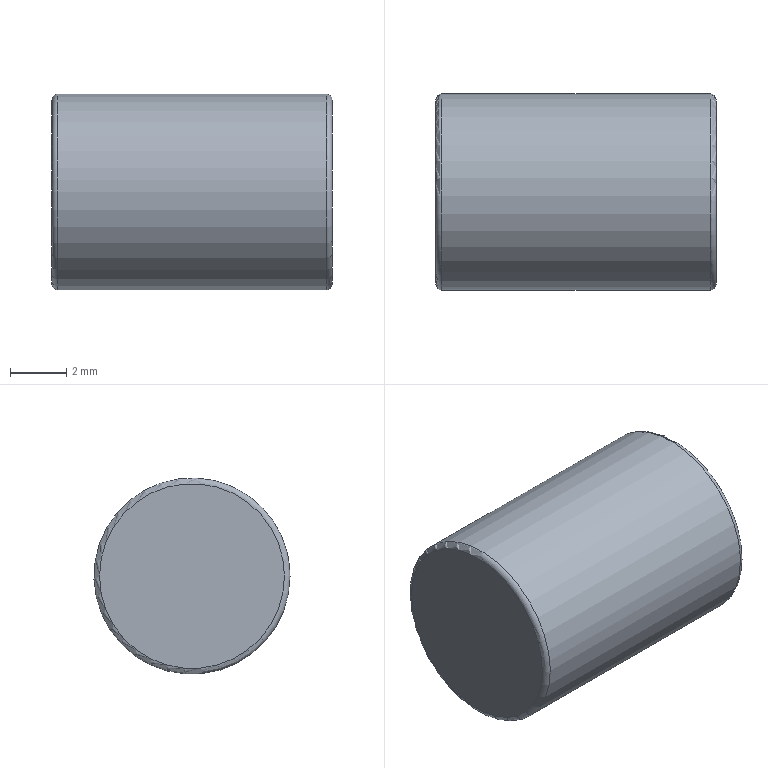Part | STEP file | Part [15] | 1 solid | 5 faces | box 10 x 7 x 7 mm | volume 384.472 mm3 | plane 2 | torus 2 | cylinder 1 | commonest cylinder face diameters 7 x1
STEP:
#1=CARTESIAN_POINT('',(-5.,-126.094,0.));
#2=VERTEX_POINT('',#1);
#3=CARTESIAN_POINT('',(-5.,-122.794,0.));
#4=DIRECTION('',(-1.,0.,0.));
#5=DIRECTION('',(0.,-1.,0.));
#6=AXIS2_PLACEMENT_3D('',#3,#4,#5);
#7=CIRCLE('',#6,3.3);
#8=EDGE_CURVE('',#2,#2,#7,.T.);
#9=ORIENTED_EDGE('',*,*,#8,.T.);
#10=EDGE_LOOP('',(#9));
#11=FACE_BOUND('',#10,.T.);
#12=CARTESIAN_POINT('',(-5.,-122.794,0.));
#13=DIRECTION('',(1.,0.,0.));
#14=DIRECTION('',(0.,0.,1.));
#15=AXIS2_PLACEMENT_3D('',#12,#13,#14);
#16=PLANE('',#15);
#17=ADVANCED_FACE('',(#11),#16,.F.);
#18=CARTESIAN_POINT('',(-4.8,-126.294,0.));
#19=VERTEX_POINT('',#18);
#20=CARTESIAN_POINT('',(-4.8,-126.294,0.));
#21=CARTESIAN_POINT('',(-4.8,-126.294,-0.07332));
#22=CARTESIAN_POINT('',(-4.8,-126.289,-0.2199));
#23=CARTESIAN_POINT('',(-4.8,-126.269,-0.439));
#24=CARTESIAN_POINT('',(-4.8,-126.234,-0.6564));
#25=CARTESIAN_POINT('',(-4.8,-126.186,-0.8711));
#26=CARTESIAN_POINT('',(-4.8,-126.125,-1.082));
#27=CARTESIAN_POINT('',(-4.8,-126.05,-1.289));
#28=CARTESIAN_POINT('',(-4.8,-125.963,-1.491));
#29=CARTESIAN_POINT('',(-4.8,-125.863,-1.687));
#30=CARTESIAN_POINT('',(-4.8,-125.751,-1.877));
#31=CARTESIAN_POINT('',(-4.8,-125.627,-2.059));
#32=CARTESIAN_POINT('',(-4.8,-125.492,-2.233));
#33=CARTESIAN_POINT('',(-4.8,-125.347,-2.398));
#34=CARTESIAN_POINT('',(-4.8,-125.191,-2.553));
#35=CARTESIAN_POINT('',(-4.8,-125.026,-2.699));
#36=CARTESIAN_POINT('',(-4.8,-124.852,-2.834));
#37=CARTESIAN_POINT('',(-4.8,-124.67,-2.957));
#38=CARTESIAN_POINT('',(-4.8,-124.481,-3.069));
#39=CARTESIAN_POINT('',(-4.8,-124.285,-3.169));
#40=CARTESIAN_POINT('',(-4.8,-124.083,-3.257));
#41=CARTESIAN_POINT('',(-4.8,-123.876,-3.331));
#42=CARTESIAN_POINT('',(-4.8,-123.664,-3.392));
#43=CARTESIAN_POINT('',(-4.8,-123.45,-3.44));
#44=CARTESIAN_POINT('',(-4.8,-123.232,-3.475));
#45=CARTESIAN_POINT('',(-4.8,-123.013,-3.495));
#46=CARTESIAN_POINT('',(-4.8,-122.793,-3.502));
#47=CARTESIAN_POINT('',(-4.8,-122.573,-3.495));
#48=CARTESIAN_POINT('',(-4.8,-122.354,-3.475));
#49=CARTESIAN_POINT('',(-4.8,-122.137,-3.44));
#50=CARTESIAN_POINT('',(-4.8,-121.922,-3.392));
#51=CARTESIAN_POINT('',(-4.8,-121.711,-3.331));
#52=CARTESIAN_POINT('',(-4.8,-121.504,-3.256));
#53=CARTESIAN_POINT('',(-4.8,-121.302,-3.169));
#54=CARTESIAN_POINT('',(-4.8,-121.106,-3.069));
#55=CARTESIAN_POINT('',(-4.8,-120.916,-2.956));
#56=CARTESIAN_POINT('',(-4.8,-120.734,-2.833));
#57=CARTESIAN_POINT('',(-4.8,-120.561,-2.698));
#58=CARTESIAN_POINT('',(-4.8,-120.396,-2.552));
#59=CARTESIAN_POINT('',(-4.8,-120.24,-2.397));
#60=CARTESIAN_POINT('',(-4.8,-120.095,-2.231));
#61=CARTESIAN_POINT('',(-4.8,-119.96,-2.057));
#62=CARTESIAN_POINT('',(-4.8,-119.836,-1.875));
#63=CARTESIAN_POINT('',(-4.8,-119.724,-1.686));
#64=CARTESIAN_POINT('',(-4.8,-119.624,-1.49));
#65=CARTESIAN_POINT('',(-4.8,-119.537,-1.288));
#66=CARTESIAN_POINT('',(-4.8,-119.463,-1.081));
#67=CARTESIAN_POINT('',(-4.8,-119.401,-0.8694));
#68=CARTESIAN_POINT('',(-4.8,-119.353,-0.6546));
#69=CARTESIAN_POINT('',(-4.8,-119.319,-0.4373));
#70=CARTESIAN_POINT('',(-4.8,-119.299,-0.2188));
#71=CARTESIAN_POINT('',(-4.8,-119.294,-0.07273));
#72=CARTESIAN_POINT('',(-4.8,-119.294,0.));
#73=CARTESIAN_POINT('',(-4.8,-119.294,0.07332));
#74=CARTESIAN_POINT('',(-4.8,-119.299,0.2199));
#75=CARTESIAN_POINT('',(-4.8,-119.319,0.439));
#76=CARTESIAN_POINT('',(-4.8,-119.354,0.6564));
#77=CARTESIAN_POINT('',(-4.8,-119.402,0.8711));
#78=CARTESIAN_POINT('',(-4.8,-119.463,1.082));
#79=CARTESIAN_POINT('',(-4.8,-119.538,1.289));
#80=CARTESIAN_POINT('',(-4.8,-119.625,1.491));
#81=CARTESIAN_POINT('',(-4.8,-119.725,1.687));
#82=CARTESIAN_POINT('',(-4.8,-119.837,1.877));
#83=CARTESIAN_POINT('',(-4.8,-119.961,2.059));
#84=CARTESIAN_POINT('',(-4.8,-120.096,2.233));
#85=CARTESIAN_POINT('',(-4.8,-120.241,2.398));
#86=CARTESIAN_POINT('',(-4.8,-120.397,2.553));
#87=CARTESIAN_POINT('',(-4.8,-120.562,2.699));
#88=CARTESIAN_POINT('',(-4.8,-120.736,2.834));
#89=CARTESIAN_POINT('',(-4.8,-120.918,2.957));
#90=CARTESIAN_POINT('',(-4.8,-121.107,3.069));
#91=CARTESIAN_POINT('',(-4.8,-121.303,3.169));
#92=CARTESIAN_POINT('',(-4.8,-121.505,3.257));
#93=CARTESIAN_POINT('',(-4.8,-121.712,3.331));
#94=CARTESIAN_POINT('',(-4.8,-121.924,3.392));
#95=CARTESIAN_POINT('',(-4.8,-122.138,3.44));
#96=CARTESIAN_POINT('',(-4.8,-122.356,3.475));
#97=CARTESIAN_POINT('',(-4.8,-122.575,3.495));
#98=CARTESIAN_POINT('',(-4.8,-122.795,3.502));
#99=CARTESIAN_POINT('',(-4.8,-123.015,3.495));
#100=CARTESIAN_POINT('',(-4.8,-123.234,3.475));
#101=CARTESIAN_POINT('',(-4.8,-123.451,3.44));
#102=CARTESIAN_POINT('',(-4.8,-123.666,3.392));
#103=CARTESIAN_POINT('',(-4.8,-123.877,3.331));
#104=CARTESIAN_POINT('',(-4.8,-124.084,3.256));
#105=CARTESIAN_POINT('',(-4.8,-124.286,3.169));
#106=CARTESIAN_POINT('',(-4.8,-124.482,3.069));
#107=CARTESIAN_POINT('',(-4.8,-124.672,2.956));
#108=CARTESIAN_POINT('',(-4.8,-124.854,2.833));
#109=CARTESIAN_POINT('',(-4.8,-125.027,2.698));
#110=CARTESIAN_POINT('',(-4.8,-125.192,2.552));
#111=CARTESIAN_POINT('',(-4.8,-125.348,2.397));
#112=CARTESIAN_POINT('',(-4.8,-125.493,2.231));
#113=CARTESIAN_POINT('',(-4.8,-125.628,2.057));
#114=CARTESIAN_POINT('',(-4.8,-125.752,1.875));
#115=CARTESIAN_POINT('',(-4.8,-125.864,1.686));
#116=CARTESIAN_POINT('',(-4.8,-125.964,1.49));
#117=CARTESIAN_POINT('',(-4.8,-126.051,1.288));
#118=CARTESIAN_POINT('',(-4.8,-126.125,1.081));
#119=CARTESIAN_POINT('',(-4.8,-126.187,0.8694));
#120=CARTESIAN_POINT('',(-4.8,-126.235,0.6546));
#121=CARTESIAN_POINT('',(-4.8,-126.269,0.4373));
#122=CARTESIAN_POINT('',(-4.8,-126.289,0.2188));
#123=CARTESIAN_POINT('',(-4.8,-126.294,0.07273));
#124=CARTESIAN_POINT('',(-4.8,-126.294,0.));
#125=B_SPLINE_CURVE_WITH_KNOTS('',3,(#20,#21,#22,#23,#24,#25,#26,#27,#28,#29,#30,#31,#32,#33,#34,#35,#36,#37,#38,#39,#40,#41,#42,#43,#44,#45,#46,#47,#48,#49,#50,#51,#52,#53,#54,#55,#56,#57,#58,#59,#60,#61,#62,#63,#64,#65,#66,#67,#68,#69,#70,#71,#72,#73,#74,#75,#76,#77,#78,#79,#80,#81,#82,#83,#84,#85,#86,#87,#88,#89,#90,#91,#92,#93,#94,#95,#96,#97,#98,#99,#100,#101,#102,#103,#104,#105,#106,#107,#108,#109,#110,#111,#112,#113,#114,#115,#116,#117,#118,#119,#120,#121,#122,#123,#124),.UNSPECIFIED.,.T.,.F.,(4,1,1,1,1,1,1,1,1,1,1,1,1,1,1,1,1,1,1,1,1,1,1,1,1,1,1,1,1,1,1,1,1,1,1,1,1,1,1,1,1,1,1,1,1,1,1,1,1,1,3,1,1,1,1,1,1,1,1,1,1,1,1,1,1,1,1,1,1,1,1,1,1,1,1,1,1,1,1,1,1,1,1,1,1,1,1,1,1,1,1,1,1,1,1,1,1,1,1,1,4),(0.,0.01,0.02,0.03,0.04001,0.05001,0.06001,0.07001,0.08001,0.09001,0.1,0.11,0.12,0.13,0.14,0.15,0.16,0.17,0.18,0.19,0.2,0.21,0.22,0.23,0.24,0.25,0.26,0.27,0.28,0.29,0.3,0.31,0.3201,0.3301,0.3401,0.3501,0.3601,0.3701,0.3801,0.3901,0.4001,0.4101,0.4201,0.4301,0.4401,0.4501,0.4601,0.4701,0.4801,0.4901,0.5,0.51,0.52,0.53,0.54,0.55,0.56,0.57,0.58,0.59,0.6,0.61,0.62,0.63,0.64,0.65,0.66,0.67,0.68,0.69,0.7,0.71,0.72,0.73,0.74,0.75,0.76,0.77,0.78,0.79,0.8,0.81,0.8201,0.8301,0.8401,0.8501,0.8601,0.8701,0.8801,0.8901,0.9001,0.9101,0.9201,0.9301,0.9401,0.9501,0.9601,0.9701,0.9801,0.9901,1.),.UNSPECIFIED.);
#126=EDGE_CURVE('',#19,#19,#125,.T.);
#127=ORIENTED_EDGE('',*,*,#126,.F.);
#128=EDGE_LOOP('',(#127));
#129=FACE_OUTER_BOUND('',#128,.T.);
#130=ORIENTED_EDGE('',*,*,#8,.F.);
#131=EDGE_LOOP('',(#130));
#132=FACE_OUTER_BOUND('',#131,.T.);
#133=CARTESIAN_POINT('',(-4.8,-122.794,0.));
#134=DIRECTION('',(1.,0.,0.));
#135=DIRECTION('',(0.,-1.,0.));
#136=AXIS2_PLACEMENT_3D('',#133,#134,#135);
#137=TOROIDAL_SURFACE('',#136,3.3,0.2);
#138=ADVANCED_FACE('',(#129,#132),#137,.T.);
#139=CARTESIAN_POINT('',(4.8,-126.294,0.));
#140=VERTEX_POINT('',#139);
#141=CARTESIAN_POINT('',(4.8,-126.294,0.));
#142=CARTESIAN_POINT('',(4.8,-126.294,-0.07332));
#143=CARTESIAN_POINT('',(4.8,-126.289,-0.2199));
#144=CARTESIAN_POINT('',(4.8,-126.269,-0.439));
#145=CARTESIAN_POINT('',(4.8,-126.234,-0.6564));
#146=CARTESIAN_POINT('',(4.8,-126.186,-0.8711));
#147=CARTESIAN_POINT('',(4.8,-126.125,-1.082));
#148=CARTESIAN_POINT('',(4.8,-126.05,-1.289));
#149=CARTESIAN_POINT('',(4.8,-125.963,-1.491));
#150=CARTESIAN_POINT('',(4.8,-125.863,-1.687));
#151=CARTESIAN_POINT('',(4.8,-125.751,-1.877));
#152=CARTESIAN_POINT('',(4.8,-125.627,-2.059));
#153=CARTESIAN_POINT('',(4.8,-125.492,-2.233));
#154=CARTESIAN_POINT('',(4.8,-125.347,-2.398));
#155=CARTESIAN_POINT('',(4.8,-125.191,-2.553));
#156=CARTESIAN_POINT('',(4.8,-125.026,-2.699));
#157=CARTESIAN_POINT('',(4.8,-124.852,-2.834));
#158=CARTESIAN_POINT('',(4.8,-124.67,-2.957));
#159=CARTESIAN_POINT('',(4.8,-124.481,-3.069));
#160=CARTESIAN_POINT('',(4.8,-124.285,-3.169));
#161=CARTESIAN_POINT('',(4.8,-124.083,-3.257));
#162=CARTESIAN_POINT('',(4.8,-123.876,-3.331));
#163=CARTESIAN_POINT('',(4.8,-123.664,-3.392));
#164=CARTESIAN_POINT('',(4.8,-123.45,-3.44));
#165=CARTESIAN_POINT('',(4.8,-123.232,-3.475));
#166=CARTESIAN_POINT('',(4.8,-123.013,-3.495));
#167=CARTESIAN_POINT('',(4.8,-122.793,-3.502));
#168=CARTESIAN_POINT('',(4.8,-122.573,-3.495));
#169=CARTESIAN_POINT('',(4.8,-122.354,-3.475));
#170=CARTESIAN_POINT('',(4.8,-122.137,-3.44));
#171=CARTESIAN_POINT('',(4.8,-121.922,-3.392));
#172=CARTESIAN_POINT('',(4.8,-121.711,-3.331));
#173=CARTESIAN_POINT('',(4.8,-121.504,-3.256));
#174=CARTESIAN_POINT('',(4.8,-121.302,-3.169));
#175=CARTESIAN_POINT('',(4.8,-121.106,-3.069));
#176=CARTESIAN_POINT('',(4.8,-120.916,-2.956));
#177=CARTESIAN_POINT('',(4.8,-120.734,-2.833));
#178=CARTESIAN_POINT('',(4.8,-120.561,-2.698));
#179=CARTESIAN_POINT('',(4.8,-120.396,-2.552));
#180=CARTESIAN_POINT('',(4.8,-120.24,-2.397));
#181=CARTESIAN_POINT('',(4.8,-120.095,-2.231));
#182=CARTESIAN_POINT('',(4.8,-119.96,-2.057));
#183=CARTESIAN_POINT('',(4.8,-119.836,-1.875));
#184=CARTESIAN_POINT('',(4.8,-119.724,-1.686));
#185=CARTESIAN_POINT('',(4.8,-119.624,-1.49));
#186=CARTESIAN_POINT('',(4.8,-119.537,-1.288));
#187=CARTESIAN_POINT('',(4.8,-119.463,-1.081));
#188=CARTESIAN_POINT('',(4.8,-119.401,-0.8694));
#189=CARTESIAN_POINT('',(4.8,-119.353,-0.6546));
#190=CARTESIAN_POINT('',(4.8,-119.319,-0.4373));
#191=CARTESIAN_POINT('',(4.8,-119.299,-0.2188));
#192=CARTESIAN_POINT('',(4.8,-119.294,-0.07273));
#193=CARTESIAN_POINT('',(4.8,-119.294,0.));
#194=CARTESIAN_POINT('',(4.8,-119.294,0.07332));
#195=CARTESIAN_POINT('',(4.8,-119.299,0.2199));
#196=CARTESIAN_POINT('',(4.8,-119.319,0.439));
#197=CARTESIAN_POINT('',(4.8,-119.354,0.6564));
#198=CARTESIAN_POINT('',(4.8,-119.402,0.8711));
#199=CARTESIAN_POINT('',(4.8,-119.463,1.082));
#200=CARTESIAN_POINT('',(4.8,-119.538,1.289));
#201=CARTESIAN_POINT('',(4.8,-119.625,1.491));
#202=CARTESIAN_POINT('',(4.8,-119.725,1.687));
#203=CARTESIAN_POINT('',(4.8,-119.837,1.877));
#204=CARTESIAN_POINT('',(4.8,-119.961,2.059));
#205=CARTESIAN_POINT('',(4.8,-120.096,2.233));
#206=CARTESIAN_POINT('',(4.8,-120.241,2.398));
#207=CARTESIAN_POINT('',(4.8,-120.397,2.553));
#208=CARTESIAN_POINT('',(4.8,-120.562,2.699));
#209=CARTESIAN_POINT('',(4.8,-120.736,2.834));
#210=CARTESIAN_POINT('',(4.8,-120.918,2.957));
#211=CARTESIAN_POINT('',(4.8,-121.107,3.069));
#212=CARTESIAN_POINT('',(4.8,-121.303,3.169));
#213=CARTESIAN_POINT('',(4.8,-121.505,3.257));
#214=CARTESIAN_POINT('',(4.8,-121.712,3.331));
#215=CARTESIAN_POINT('',(4.8,-121.924,3.392));
#216=CARTESIAN_POINT('',(4.8,-122.138,3.44));
#217=CARTESIAN_POINT('',(4.8,-122.356,3.475));
#218=CARTESIAN_POINT('',(4.8,-122.575,3.495));
#219=CARTESIAN_POINT('',(4.8,-122.795,3.502));
#220=CARTESIAN_POINT('',(4.8,-123.015,3.495));
#221=CARTESIAN_POINT('',(4.8,-123.234,3.475));
#222=CARTESIAN_POINT('',(4.8,-123.451,3.44));
#223=CARTESIAN_POINT('',(4.8,-123.666,3.392));
#224=CARTESIAN_POINT('',(4.8,-123.877,3.331));
#225=CARTESIAN_POINT('',(4.8,-124.084,3.256));
#226=CARTESIAN_POINT('',(4.8,-124.286,3.169));
#227=CARTESIAN_POINT('',(4.8,-124.482,3.069));
#228=CARTESIAN_POINT('',(4.8,-124.672,2.956));
#229=CARTESIAN_POINT('',(4.8,-124.854,2.833));
#230=CARTESIAN_POINT('',(4.8,-125.027,2.698));
#231=CARTESIAN_POINT('',(4.8,-125.192,2.552));
#232=CARTESIAN_POINT('',(4.8,-125.348,2.397));
#233=CARTESIAN_POINT('',(4.8,-125.493,2.231));
#234=CARTESIAN_POINT('',(4.8,-125.628,2.057));
#235=CARTESIAN_POINT('',(4.8,-125.752,1.875));
#236=CARTESIAN_POINT('',(4.8,-125.864,1.686));
#237=CARTESIAN_POINT('',(4.8,-125.964,1.49));
#238=CARTESIAN_POINT('',(4.8,-126.051,1.288));
#239=CARTESIAN_POINT('',(4.8,-126.125,1.081));
#240=CARTESIAN_POINT('',(4.8,-126.187,0.8694));
#241=CARTESIAN_POINT('',(4.8,-126.235,0.6546));
#242=CARTESIAN_POINT('',(4.8,-126.269,0.4373));
#243=CARTESIAN_POINT('',(4.8,-126.289,0.2188));
#244=CARTESIAN_POINT('',(4.8,-126.294,0.07273));
#245=CARTESIAN_POINT('',(4.8,-126.294,0.));
#246=B_SPLINE_CURVE_WITH_KNOTS('',3,(#141,#142,#143,#144,#145,#146,#147,#148,#149,#150,#151,#152,#153,#154,#155,#156,#157,#158,#159,#160,#161,#162,#163,#164,#165,#166,#167,#168,#169,#170,#171,#172,#173,#174,#175,#176,#177,#178,#179,#180,#181,#182,#183,#184,#185,#186,#187,#188,#189,#190,#191,#192,#193,#194,#195,#196,#197,#198,#199,#200,#201,#202,#203,#204,#205,#206,#207,#208,#209,#210,#211,#212,#213,#214,#215,#216,#217,#218,#219,#220,#221,#222,#223,#224,#225,#226,#227,#228,#229,#230,#231,#232,#233,#234,#235,#236,#237,#238,#239,#240,#241,#242,#243,#244,#245),.UNSPECIFIED.,.T.,.F.,(4,1,1,1,1,1,1,1,1,1,1,1,1,1,1,1,1,1,1,1,1,1,1,1,1,1,1,1,1,1,1,1,1,1,1,1,1,1,1,1,1,1,1,1,1,1,1,1,1,1,3,1,1,1,1,1,1,1,1,1,1,1,1,1,1,1,1,1,1,1,1,1,1,1,1,1,1,1,1,1,1,1,1,1,1,1,1,1,1,1,1,1,1,1,1,1,1,1,1,1,4),(0.,0.01,0.02,0.03,0.04001,0.05001,0.06001,0.07001,0.08001,0.09001,0.1,0.11,0.12,0.13,0.14,0.15,0.16,0.17,0.18,0.19,0.2,0.21,0.22,0.23,0.24,0.25,0.26,0.27,0.28,0.29,0.3,0.31,0.3201,0.3301,0.3401,0.3501,0.3601,0.3701,0.3801,0.3901,0.4001,0.4101,0.4201,0.4301,0.4401,0.4501,0.4601,0.4701,0.4801,0.4901,0.5,0.51,0.52,0.53,0.54,0.55,0.56,0.57,0.58,0.59,0.6,0.61,0.62,0.63,0.64,0.65,0.66,0.67,0.68,0.69,0.7,0.71,0.72,0.73,0.74,0.75,0.76,0.77,0.78,0.79,0.8,0.81,0.8201,0.8301,0.8401,0.8501,0.8601,0.8701,0.8801,0.8901,0.9001,0.9101,0.9201,0.9301,0.9401,0.9501,0.9601,0.9701,0.9801,0.9901,1.),.UNSPECIFIED.);
#247=EDGE_CURVE('',#140,#140,#246,.T.);
#248=ORIENTED_EDGE('',*,*,#247,.F.);
#249=EDGE_LOOP('',(#248));
#250=FACE_OUTER_BOUND('',#249,.T.);
#251=ORIENTED_EDGE('',*,*,#126,.T.);
#252=EDGE_LOOP('',(#251));
#253=FACE_OUTER_BOUND('',#252,.T.);
#254=CARTESIAN_POINT('',(-5.5,-122.794,0.));
#255=DIRECTION('',(1.,0.,0.));
#256=DIRECTION('',(0.,-1.,0.));
#257=AXIS2_PLACEMENT_3D('',#254,#255,#256);
#258=CYLINDRICAL_SURFACE('',#257,3.5);
#259=ADVANCED_FACE('',(#250,#253),#258,.T.);
#260=CARTESIAN_POINT('',(5.,-126.094,0.));
#261=VERTEX_POINT('',#260);
#262=CARTESIAN_POINT('',(5.,-122.794,0.));
#263=DIRECTION('',(1.,0.,0.));
#264=DIRECTION('',(0.,-1.,0.));
#265=AXIS2_PLACEMENT_3D('',#262,#263,#264);
#266=CIRCLE('',#265,3.3);
#267=EDGE_CURVE('',#261,#261,#266,.T.);
#268=ORIENTED_EDGE('',*,*,#267,.F.);
#269=EDGE_LOOP('',(#268));
#270=FACE_OUTER_BOUND('',#269,.T.);
#271=ORIENTED_EDGE('',*,*,#247,.T.);
#272=EDGE_LOOP('',(#271));
#273=FACE_OUTER_BOUND('',#272,.T.);
#274=CARTESIAN_POINT('',(4.8,-122.794,0.));
#275=DIRECTION('',(1.,0.,0.));
#276=DIRECTION('',(0.,-1.,0.));
#277=AXIS2_PLACEMENT_3D('',#274,#275,#276);
#278=TOROIDAL_SURFACE('',#277,3.3,0.2);
#279=ADVANCED_FACE('',(#270,#273),#278,.T.);
#280=ORIENTED_EDGE('',*,*,#267,.T.);
#281=EDGE_LOOP('',(#280));
#282=FACE_BOUND('',#281,.T.);
#283=CARTESIAN_POINT('',(5.,-122.794,0.));
#284=DIRECTION('',(1.,0.,0.));
#285=DIRECTION('',(0.,0.,1.));
#286=AXIS2_PLACEMENT_3D('',#283,#284,#285);
#287=PLANE('',#286);
#288=ADVANCED_FACE('',(#282),#287,.T.);
#289=CLOSED_SHELL('',(#17,#138,#259,#279,#288));
#290=MANIFOLD_SOLID_BREP('',#289);
#291=(LENGTH_UNIT()NAMED_UNIT(*)SI_UNIT(.MILLI.,.METRE.));
#292=UNCERTAINTY_MEASURE_WITH_UNIT(LENGTH_MEASURE(0.00001),#291,'','');
#293=(NAMED_UNIT(*)PLANE_ANGLE_UNIT()SI_UNIT($,.RADIAN.));
#294=(NAMED_UNIT(*)SI_UNIT($,.STERADIAN.)SOLID_ANGLE_UNIT());
#295=(GEOMETRIC_REPRESENTATION_CONTEXT(3)GLOBAL_UNCERTAINTY_ASSIGNED_CONTEXT((#292))GLOBAL_UNIT_ASSIGNED_CONTEXT((#291,#293,#294))REPRESENTATION_CONTEXT('',''));
#296=ADVANCED_BREP_SHAPE_REPRESENTATION('',(#290),#295);